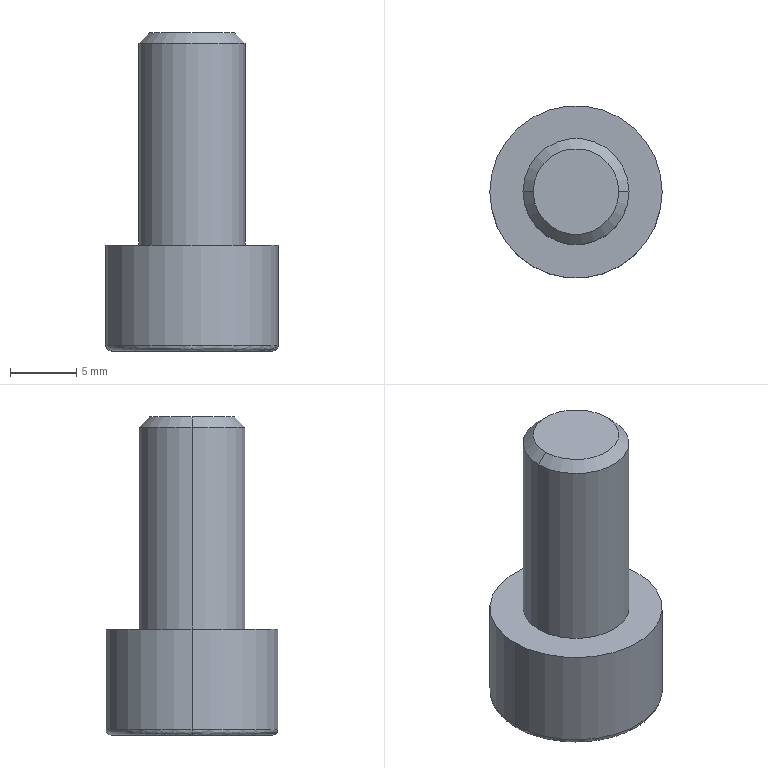Part | STEP file | 10 | 1 solid | 19 faces | box 13 x 13 x 24 mm | volume 1690 mm3 | plane 9 | cylinder 4 | cone 4 | spline 2 | commonest cylinder face diameters 8 x2 13 x2